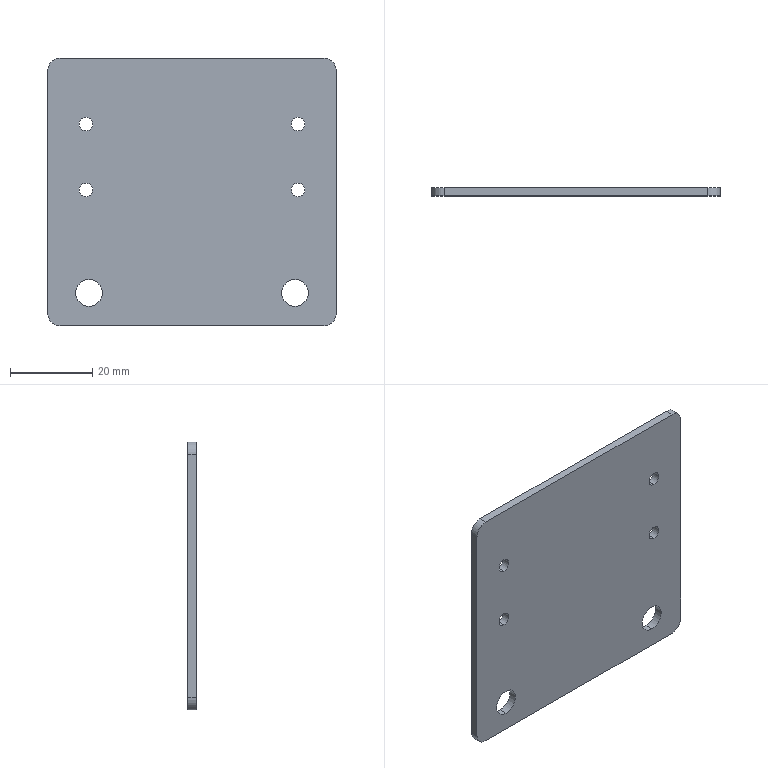Part | STEP file | Solenoid Valve Mounting Adapter Plate | 1 solid | 22 faces | box 70 x 2 x 65 mm | volume 8883 mm3 | cylinder 16 | plane 6 | commonest cylinder face diameters 3.3 x8 6 x4 6.5 x4